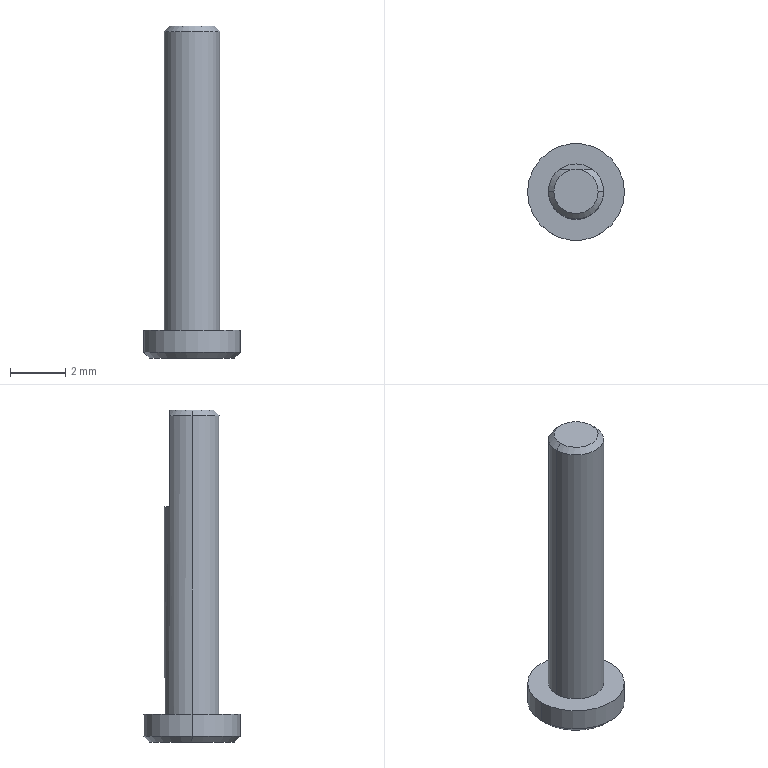Part | SolidWorks | features ICE 2, Chamfer 1, Extrusion 1 | 1 solid | 14 faces | box 3.5 x 3.5 x 12 mm | volume 43.298 mm3 | cone 5 | plane 5 | cylinder 4 | commonest cylinder face diameters 2 x2 3.5 x2
STEP:
#1=CARTESIAN_POINT('',(0.8,0.,12.));
#2=VERTEX_POINT('',#1);
#3=CARTESIAN_POINT('',(0.,0.8,12.));
#4=VERTEX_POINT('',#3);
#5=CARTESIAN_POINT('',(0.,0.,12.));
#6=DIRECTION('',(0.,0.,1.));
#7=DIRECTION('',(1.,0.,0.));
#8=AXIS2_PLACEMENT_3D('',#5,#6,#7);
#9=CIRCLE('',#8,0.8);
#10=EDGE_CURVE('',#2,#4,#9,.T.);
#11=ORIENTED_EDGE('',*,*,#10,.F.);
#12=CARTESIAN_POINT('',(1.,0.,11.8));
#13=VERTEX_POINT('',#12);
#14=CARTESIAN_POINT('',(0.8,0.,12.));
#15=DIRECTION('',(0.7071,0.,-0.7071));
#16=VECTOR('',#15,1000.);
#17=LINE('',#14,#16);
#18=EDGE_CURVE('',#2,#13,#17,.T.);
#19=ORIENTED_EDGE('',*,*,#18,.T.);
#20=CARTESIAN_POINT('',(0.6,0.8,11.8));
#21=VERTEX_POINT('',#20);
#22=CARTESIAN_POINT('',(0.,0.,11.8));
#23=DIRECTION('',(0.,0.,-1.));
#24=DIRECTION('',(1.,0.,0.));
#25=AXIS2_PLACEMENT_3D('',#22,#23,#24);
#26=CIRCLE('',#25,1.);
#27=EDGE_CURVE('',#21,#13,#26,.T.);
#28=ORIENTED_EDGE('',*,*,#27,.F.);
#29=CARTESIAN_POINT('',(0.,0.8,12.));
#30=CARTESIAN_POINT('',(0.1071,0.8,12.));
#31=CARTESIAN_POINT('',(0.2131,0.8,11.977));
#32=CARTESIAN_POINT('',(0.414,0.8,11.904));
#33=CARTESIAN_POINT('',(0.5084,0.8,11.855));
#34=CARTESIAN_POINT('',(0.6,0.8,11.8));
#35=B_SPLINE_CURVE_WITH_KNOTS('',3,(#29,#30,#31,#32,#33,#34),.UNSPECIFIED.,.F.,.F.,(4,2,4),(0.001408,0.001725,0.002043),.UNSPECIFIED.);
#36=EDGE_CURVE('',#4,#21,#35,.T.);
#37=ORIENTED_EDGE('',*,*,#36,.F.);
#38=EDGE_LOOP('',(#11,#19,#28,#37));
#39=FACE_OUTER_BOUND('',#38,.T.);
#40=CARTESIAN_POINT('',(0.,0.,12.));
#41=DIRECTION('',(0.,0.,-1.));
#42=DIRECTION('',(-1.,0.,0.));
#43=AXIS2_PLACEMENT_3D('',#40,#41,#42);
#44=CONICAL_SURFACE('',#43,0.8,0.7854);
#45=ADVANCED_FACE('',(#39),#44,.T.);
#46=ORIENTED_EDGE('',*,*,#18,.F.);
#47=CARTESIAN_POINT('',(-0.8,0.,12.));
#48=VERTEX_POINT('',#47);
#49=CARTESIAN_POINT('',(0.,0.,12.));
#50=DIRECTION('',(0.,0.,1.));
#51=DIRECTION('',(1.,0.,0.));
#52=AXIS2_PLACEMENT_3D('',#49,#50,#51);
#53=CIRCLE('',#52,0.8);
#54=EDGE_CURVE('',#48,#2,#53,.T.);
#55=ORIENTED_EDGE('',*,*,#54,.F.);
#56=CARTESIAN_POINT('',(-1.,0.,11.8));
#57=VERTEX_POINT('',#56);
#58=CARTESIAN_POINT('',(-0.8,0.,12.));
#59=DIRECTION('',(-0.7071,0.,-0.7071));
#60=VECTOR('',#59,1000.);
#61=LINE('',#58,#60);
#62=EDGE_CURVE('',#48,#57,#61,.T.);
#63=ORIENTED_EDGE('',*,*,#62,.T.);
#64=CARTESIAN_POINT('',(0.,0.,11.8));
#65=DIRECTION('',(0.,0.,-1.));
#66=DIRECTION('',(1.,0.,0.));
#67=AXIS2_PLACEMENT_3D('',#64,#65,#66);
#68=CIRCLE('',#67,1.);
#69=EDGE_CURVE('',#13,#57,#68,.T.);
#70=ORIENTED_EDGE('',*,*,#69,.F.);
#71=EDGE_LOOP('',(#46,#55,#63,#70));
#72=FACE_OUTER_BOUND('',#71,.T.);
#73=CARTESIAN_POINT('',(0.,0.,12.));
#74=DIRECTION('',(0.,0.,-1.));
#75=DIRECTION('',(-1.,0.,0.));
#76=AXIS2_PLACEMENT_3D('',#73,#74,#75);
#77=CONICAL_SURFACE('',#76,0.8,0.7854);
#78=ADVANCED_FACE('',(#72),#77,.T.);
#79=CARTESIAN_POINT('',(-1.55,0.,0.));
#80=VERTEX_POINT('',#79);
#81=CARTESIAN_POINT('',(1.55,0.,0.));
#82=VERTEX_POINT('',#81);
#83=CARTESIAN_POINT('',(0.,0.,0.));
#84=DIRECTION('',(0.,0.,-1.));
#85=DIRECTION('',(1.,0.,0.));
#86=AXIS2_PLACEMENT_3D('',#83,#84,#85);
#87=CIRCLE('',#86,1.55);
#88=EDGE_CURVE('',#80,#82,#87,.T.);
#89=ORIENTED_EDGE('',*,*,#88,.F.);
#90=CARTESIAN_POINT('',(-1.75,0.,0.2));
#91=VERTEX_POINT('',#90);
#92=CARTESIAN_POINT('',(-1.75,0.,0.2));
#93=DIRECTION('',(-0.7071,0.,0.7071));
#94=VECTOR('',#93,1000.);
#95=LINE('',#92,#94);
#96=EDGE_CURVE('',#80,#91,#95,.T.);
#97=ORIENTED_EDGE('',*,*,#96,.T.);
#98=CARTESIAN_POINT('',(1.75,0.,0.2));
#99=VERTEX_POINT('',#98);
#100=CARTESIAN_POINT('',(0.,0.,0.2));
#101=DIRECTION('',(0.,0.,1.));
#102=DIRECTION('',(1.,0.,0.));
#103=AXIS2_PLACEMENT_3D('',#100,#101,#102);
#104=CIRCLE('',#103,1.75);
#105=EDGE_CURVE('',#99,#91,#104,.T.);
#106=ORIENTED_EDGE('',*,*,#105,.F.);
#107=CARTESIAN_POINT('',(1.75,0.,0.2));
#108=DIRECTION('',(0.7071,0.,0.7071));
#109=VECTOR('',#108,1000.);
#110=LINE('',#107,#109);
#111=EDGE_CURVE('',#82,#99,#110,.T.);
#112=ORIENTED_EDGE('',*,*,#111,.F.);
#113=EDGE_LOOP('',(#89,#97,#106,#112));
#114=FACE_OUTER_BOUND('',#113,.T.);
#115=CARTESIAN_POINT('',(0.,0.,0.2));
#116=DIRECTION('',(0.,0.,1.));
#117=DIRECTION('',(1.,0.,0.));
#118=AXIS2_PLACEMENT_3D('',#115,#116,#117);
#119=CONICAL_SURFACE('',#118,1.75,0.7854);
#120=ADVANCED_FACE('',(#114),#119,.T.);
#121=ORIENTED_EDGE('',*,*,#27,.T.);
#122=CARTESIAN_POINT('',(1.,0.,1.));
#123=VERTEX_POINT('',#122);
#124=CARTESIAN_POINT('',(1.,0.,12.));
#125=DIRECTION('',(0.,0.,-1.));
#126=VECTOR('',#125,1000.);
#127=LINE('',#124,#126);
#128=EDGE_CURVE('',#13,#123,#127,.T.);
#129=ORIENTED_EDGE('',*,*,#128,.T.);
#130=CARTESIAN_POINT('',(-1.,0.,1.));
#131=VERTEX_POINT('',#130);
#132=CARTESIAN_POINT('',(0.,0.,1.));
#133=DIRECTION('',(0.,0.,1.));
#134=DIRECTION('',(1.,0.,0.));
#135=AXIS2_PLACEMENT_3D('',#132,#133,#134);
#136=CIRCLE('',#135,1.);
#137=EDGE_CURVE('',#123,#131,#136,.T.);
#138=ORIENTED_EDGE('',*,*,#137,.T.);
#139=CARTESIAN_POINT('',(-1.,0.,12.));
#140=DIRECTION('',(0.,0.,-1.));
#141=VECTOR('',#140,1000.);
#142=LINE('',#139,#141);
#143=EDGE_CURVE('',#57,#131,#142,.T.);
#144=ORIENTED_EDGE('',*,*,#143,.F.);
#145=CARTESIAN_POINT('',(-0.6,0.8,11.8));
#146=VERTEX_POINT('',#145);
#147=CARTESIAN_POINT('',(0.,0.,11.8));
#148=DIRECTION('',(0.,0.,-1.));
#149=DIRECTION('',(1.,0.,0.));
#150=AXIS2_PLACEMENT_3D('',#147,#148,#149);
#151=CIRCLE('',#150,1.);
#152=EDGE_CURVE('',#57,#146,#151,.T.);
#153=ORIENTED_EDGE('',*,*,#152,.T.);
#154=CARTESIAN_POINT('',(-0.6,0.8,8.5));
#155=VERTEX_POINT('',#154);
#156=CARTESIAN_POINT('',(-0.6,0.8,8.5));
#157=DIRECTION('',(0.,0.,1.));
#158=VECTOR('',#157,1000.);
#159=LINE('',#156,#158);
#160=EDGE_CURVE('',#155,#146,#159,.T.);
#161=ORIENTED_EDGE('',*,*,#160,.F.);
#162=CARTESIAN_POINT('',(0.6,0.8,8.5));
#163=VERTEX_POINT('',#162);
#164=CARTESIAN_POINT('',(0.,0.,8.5));
#165=DIRECTION('',(0.,0.,1.));
#166=DIRECTION('',(1.,0.,0.));
#167=AXIS2_PLACEMENT_3D('',#164,#165,#166);
#168=CIRCLE('',#167,1.);
#169=EDGE_CURVE('',#163,#155,#168,.T.);
#170=ORIENTED_EDGE('',*,*,#169,.F.);
#171=CARTESIAN_POINT('',(0.6,0.8,8.5));
#172=DIRECTION('',(0.,0.,1.));
#173=VECTOR('',#172,1000.);
#174=LINE('',#171,#173);
#175=EDGE_CURVE('',#163,#21,#174,.T.);
#176=ORIENTED_EDGE('',*,*,#175,.T.);
#177=EDGE_LOOP('',(#121,#129,#138,#144,#153,#161,#170,#176));
#178=FACE_OUTER_BOUND('',#177,.T.);
#179=CARTESIAN_POINT('',(0.,0.,12.));
#180=DIRECTION('',(0.,0.,-1.));
#181=DIRECTION('',(-1.,0.,0.));
#182=AXIS2_PLACEMENT_3D('',#179,#180,#181);
#183=CYLINDRICAL_SURFACE('',#182,1.);
#184=ADVANCED_FACE('',(#178),#183,.T.);
#185=CARTESIAN_POINT('',(1.75,0.,1.));
#186=VERTEX_POINT('',#185);
#187=CARTESIAN_POINT('',(-1.75,0.,1.));
#188=VERTEX_POINT('',#187);
#189=CARTESIAN_POINT('',(0.,0.,1.));
#190=DIRECTION('',(0.,0.,1.));
#191=DIRECTION('',(1.,0.,0.));
#192=AXIS2_PLACEMENT_3D('',#189,#190,#191);
#193=CIRCLE('',#192,1.75);
#194=EDGE_CURVE('',#186,#188,#193,.T.);
#195=ORIENTED_EDGE('',*,*,#194,.F.);
#196=CARTESIAN_POINT('',(1.75,0.,1.));
#197=DIRECTION('',(0.,0.,-1.));
#198=VECTOR('',#197,1000.);
#199=LINE('',#196,#198);
#200=EDGE_CURVE('',#186,#99,#199,.T.);
#201=ORIENTED_EDGE('',*,*,#200,.T.);
#202=ORIENTED_EDGE('',*,*,#105,.T.);
#203=CARTESIAN_POINT('',(-1.75,0.,1.));
#204=DIRECTION('',(0.,0.,-1.));
#205=VECTOR('',#204,1000.);
#206=LINE('',#203,#205);
#207=EDGE_CURVE('',#188,#91,#206,.T.);
#208=ORIENTED_EDGE('',*,*,#207,.F.);
#209=EDGE_LOOP('',(#195,#201,#202,#208));
#210=FACE_OUTER_BOUND('',#209,.T.);
#211=CARTESIAN_POINT('',(0.,0.,1.));
#212=DIRECTION('',(0.,0.,-1.));
#213=DIRECTION('',(-1.,0.,0.));
#214=AXIS2_PLACEMENT_3D('',#211,#212,#213);
#215=CYLINDRICAL_SURFACE('',#214,1.75);
#216=ADVANCED_FACE('',(#210),#215,.T.);
#217=CARTESIAN_POINT('',(0.,0.,1.));
#218=DIRECTION('',(0.,0.,1.));
#219=DIRECTION('',(1.,0.,0.));
#220=AXIS2_PLACEMENT_3D('',#217,#218,#219);
#221=CIRCLE('',#220,1.75);
#222=EDGE_CURVE('',#188,#186,#221,.T.);
#223=ORIENTED_EDGE('',*,*,#222,.T.);
#224=ORIENTED_EDGE('',*,*,#194,.T.);
#225=EDGE_LOOP('',(#223,#224));
#226=FACE_OUTER_BOUND('',#225,.T.);
#227=CARTESIAN_POINT('',(0.,0.,1.));
#228=DIRECTION('',(0.,0.,1.));
#229=DIRECTION('',(1.,0.,0.));
#230=AXIS2_PLACEMENT_3D('',#227,#228,#229);
#231=CIRCLE('',#230,1.);
#232=EDGE_CURVE('',#131,#123,#231,.T.);
#233=ORIENTED_EDGE('',*,*,#232,.F.);
#234=ORIENTED_EDGE('',*,*,#137,.F.);
#235=EDGE_LOOP('',(#233,#234));
#236=FACE_BOUND('',#235,.T.);
#237=CARTESIAN_POINT('',(0.,0.,1.));
#238=DIRECTION('',(0.,0.,1.));
#239=DIRECTION('',(1.,0.,0.));
#240=AXIS2_PLACEMENT_3D('',#237,#238,#239);
#241=PLANE('',#240);
#242=ADVANCED_FACE('',(#226,#236),#241,.T.);
#243=ORIENTED_EDGE('',*,*,#200,.F.);
#244=ORIENTED_EDGE('',*,*,#222,.F.);
#245=ORIENTED_EDGE('',*,*,#207,.T.);
#246=CARTESIAN_POINT('',(0.,0.,0.2));
#247=DIRECTION('',(0.,0.,1.));
#248=DIRECTION('',(1.,0.,0.));
#249=AXIS2_PLACEMENT_3D('',#246,#247,#248);
#250=CIRCLE('',#249,1.75);
#251=EDGE_CURVE('',#91,#99,#250,.T.);
#252=ORIENTED_EDGE('',*,*,#251,.T.);
#253=EDGE_LOOP('',(#243,#244,#245,#252));
#254=FACE_OUTER_BOUND('',#253,.T.);
#255=CARTESIAN_POINT('',(0.,0.,1.));
#256=DIRECTION('',(0.,0.,-1.));
#257=DIRECTION('',(-1.,0.,0.));
#258=AXIS2_PLACEMENT_3D('',#255,#256,#257);
#259=CYLINDRICAL_SURFACE('',#258,1.75);
#260=ADVANCED_FACE('',(#254),#259,.T.);
#261=CARTESIAN_POINT('',(0.,0.,0.));
#262=DIRECTION('',(0.,0.,-1.));
#263=DIRECTION('',(1.,0.,0.));
#264=AXIS2_PLACEMENT_3D('',#261,#262,#263);
#265=CIRCLE('',#264,1.55);
#266=EDGE_CURVE('',#82,#80,#265,.T.);
#267=ORIENTED_EDGE('',*,*,#266,.T.);
#268=ORIENTED_EDGE('',*,*,#88,.T.);
#269=EDGE_LOOP('',(#267,#268));
#270=FACE_OUTER_BOUND('',#269,.T.);
#271=CARTESIAN_POINT('',(0.,0.,0.));
#272=DIRECTION('',(0.,0.,1.));
#273=DIRECTION('',(1.,0.,0.));
#274=AXIS2_PLACEMENT_3D('',#271,#272,#273);
#275=PLANE('',#274);
#276=ADVANCED_FACE('',(#270),#275,.F.);
#277=ORIENTED_EDGE('',*,*,#128,.F.);
#278=ORIENTED_EDGE('',*,*,#69,.T.);
#279=ORIENTED_EDGE('',*,*,#143,.T.);
#280=ORIENTED_EDGE('',*,*,#232,.T.);
#281=EDGE_LOOP('',(#277,#278,#279,#280));
#282=FACE_OUTER_BOUND('',#281,.T.);
#283=CARTESIAN_POINT('',(0.,0.,12.));
#284=DIRECTION('',(0.,0.,-1.));
#285=DIRECTION('',(-1.,0.,0.));
#286=AXIS2_PLACEMENT_3D('',#283,#284,#285);
#287=CYLINDRICAL_SURFACE('',#286,1.);
#288=ADVANCED_FACE('',(#282),#287,.T.);
#289=CARTESIAN_POINT('',(0.,0.,12.));
#290=DIRECTION('',(0.,0.,1.));
#291=DIRECTION('',(1.,0.,0.));
#292=AXIS2_PLACEMENT_3D('',#289,#290,#291);
#293=CIRCLE('',#292,0.8);
#294=EDGE_CURVE('',#4,#48,#293,.T.);
#295=ORIENTED_EDGE('',*,*,#294,.T.);
#296=ORIENTED_EDGE('',*,*,#54,.T.);
#297=ORIENTED_EDGE('',*,*,#10,.T.);
#298=EDGE_LOOP('',(#295,#296,#297));
#299=FACE_OUTER_BOUND('',#298,.T.);
#300=CARTESIAN_POINT('',(0.,0.,12.));
#301=DIRECTION('',(0.,0.,1.));
#302=DIRECTION('',(1.,0.,0.));
#303=AXIS2_PLACEMENT_3D('',#300,#301,#302);
#304=PLANE('',#303);
#305=ADVANCED_FACE('',(#299),#304,.T.);
#306=ORIENTED_EDGE('',*,*,#96,.F.);
#307=ORIENTED_EDGE('',*,*,#266,.F.);
#308=ORIENTED_EDGE('',*,*,#111,.T.);
#309=ORIENTED_EDGE('',*,*,#251,.F.);
#310=EDGE_LOOP('',(#306,#307,#308,#309));
#311=FACE_OUTER_BOUND('',#310,.T.);
#312=CARTESIAN_POINT('',(0.,0.,0.2));
#313=DIRECTION('',(0.,0.,1.));
#314=DIRECTION('',(1.,0.,0.));
#315=AXIS2_PLACEMENT_3D('',#312,#313,#314);
#316=CONICAL_SURFACE('',#315,1.75,0.7854);
#317=ADVANCED_FACE('',(#311),#316,.T.);
#318=ORIENTED_EDGE('',*,*,#62,.F.);
#319=ORIENTED_EDGE('',*,*,#294,.F.);
#320=CARTESIAN_POINT('',(-0.6,0.8,11.8));
#321=CARTESIAN_POINT('',(-0.5088,0.8,11.855));
#322=CARTESIAN_POINT('',(-0.4127,0.8,11.905));
#323=CARTESIAN_POINT('',(-0.2132,0.8,11.977));
#324=CARTESIAN_POINT('',(-0.1073,0.8,12.));
#325=CARTESIAN_POINT('',(0.,0.8,12.));
#326=B_SPLINE_CURVE_WITH_KNOTS('',3,(#320,#321,#322,#323,#324,#325),.UNSPECIFIED.,.F.,.F.,(4,2,4),(0.0007713,0.00109,0.001408),.UNSPECIFIED.);
#327=EDGE_CURVE('',#146,#4,#326,.T.);
#328=ORIENTED_EDGE('',*,*,#327,.F.);
#329=ORIENTED_EDGE('',*,*,#152,.F.);
#330=EDGE_LOOP('',(#318,#319,#328,#329));
#331=FACE_OUTER_BOUND('',#330,.T.);
#332=CARTESIAN_POINT('',(0.,0.,12.));
#333=DIRECTION('',(0.,0.,-1.));
#334=DIRECTION('',(-1.,0.,0.));
#335=AXIS2_PLACEMENT_3D('',#332,#333,#334);
#336=CONICAL_SURFACE('',#335,0.8,0.7854);
#337=ADVANCED_FACE('',(#331),#336,.T.);
#338=ORIENTED_EDGE('',*,*,#327,.T.);
#339=ORIENTED_EDGE('',*,*,#36,.T.);
#340=ORIENTED_EDGE('',*,*,#175,.F.);
#341=CARTESIAN_POINT('',(-0.6,0.8,8.5));
#342=DIRECTION('',(1.,0.,0.));
#343=VECTOR('',#342,1000.);
#344=LINE('',#341,#343);
#345=EDGE_CURVE('',#155,#163,#344,.T.);
#346=ORIENTED_EDGE('',*,*,#345,.F.);
#347=ORIENTED_EDGE('',*,*,#160,.T.);
#348=EDGE_LOOP('',(#338,#339,#340,#346,#347));
#349=FACE_OUTER_BOUND('',#348,.T.);
#350=CARTESIAN_POINT('',(-0.6,0.8,8.5));
#351=DIRECTION('',(0.,-1.,0.));
#352=DIRECTION('',(0.,0.,-1.));
#353=AXIS2_PLACEMENT_3D('',#350,#351,#352);
#354=PLANE('',#353);
#355=ADVANCED_FACE('',(#349),#354,.F.);
#356=ORIENTED_EDGE('',*,*,#169,.T.);
#357=ORIENTED_EDGE('',*,*,#345,.T.);
#358=EDGE_LOOP('',(#356,#357));
#359=FACE_OUTER_BOUND('',#358,.T.);
#360=CARTESIAN_POINT('',(0.,0.,8.5));
#361=DIRECTION('',(0.,0.,1.));
#362=DIRECTION('',(1.,0.,0.));
#363=AXIS2_PLACEMENT_3D('',#360,#361,#362);
#364=PLANE('',#363);
#365=ADVANCED_FACE('',(#359),#364,.T.);
#366=CLOSED_SHELL('',(#45,#78,#120,#184,#216,#242,#260,#276,#288,#305,#317,#337,#355,#365));
#367=MANIFOLD_SOLID_BREP('',#366);
#368=CARTESIAN_POINT('',(0.,0.,0.));
#369=DIRECTION('',(0.,0.,1.));
#370=DIRECTION('',(1.,0.,0.));
#371=AXIS2_PLACEMENT_3D('',#368,#369,#370);
#372=(LENGTH_UNIT()NAMED_UNIT(*)SI_UNIT(.MILLI.,.METRE.));
#373=UNCERTAINTY_MEASURE_WITH_UNIT(LENGTH_MEASURE(0.00001),#372,'','');
#374=(NAMED_UNIT(*)PLANE_ANGLE_UNIT()SI_UNIT($,.RADIAN.));
#375=(NAMED_UNIT(*)SI_UNIT($,.STERADIAN.)SOLID_ANGLE_UNIT());
#376=(GEOMETRIC_REPRESENTATION_CONTEXT(3)GLOBAL_UNCERTAINTY_ASSIGNED_CONTEXT((#373))GLOBAL_UNIT_ASSIGNED_CONTEXT((#372,#374,#375))REPRESENTATION_CONTEXT('',''));
#377=ADVANCED_BREP_SHAPE_REPRESENTATION('',(#367,#371),#376);